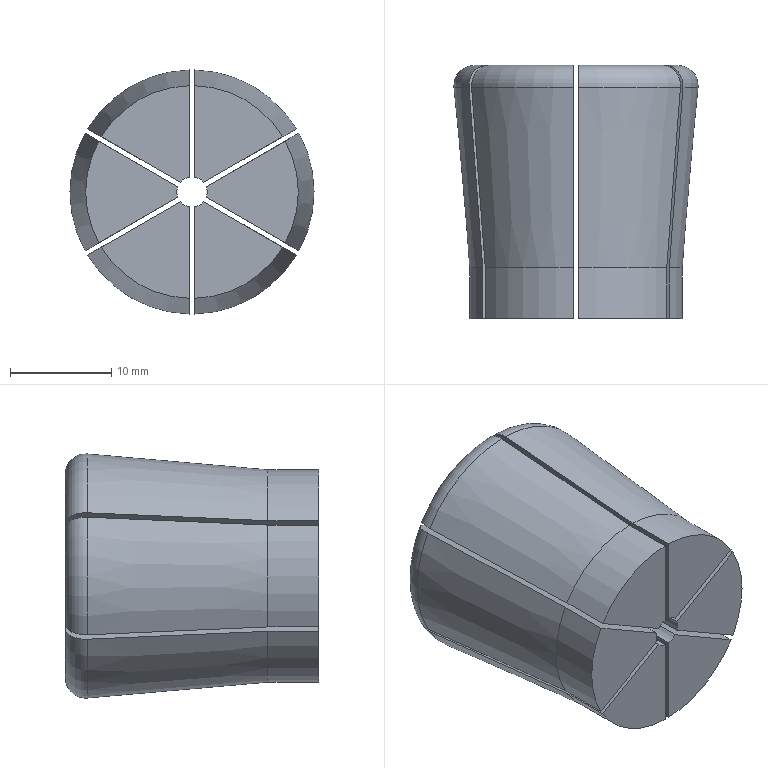Part | SolidWorks | features ICE 4, RefAxis 1, Revolution 1 | 6 solids | 48 faces | box 24.134 x 25 x 24.129 mm | volume 8899 mm3 | plane 24 | cylinder 12 | cone 6 | torus 6 | commonest cylinder face diameters 3 x6 21 x6